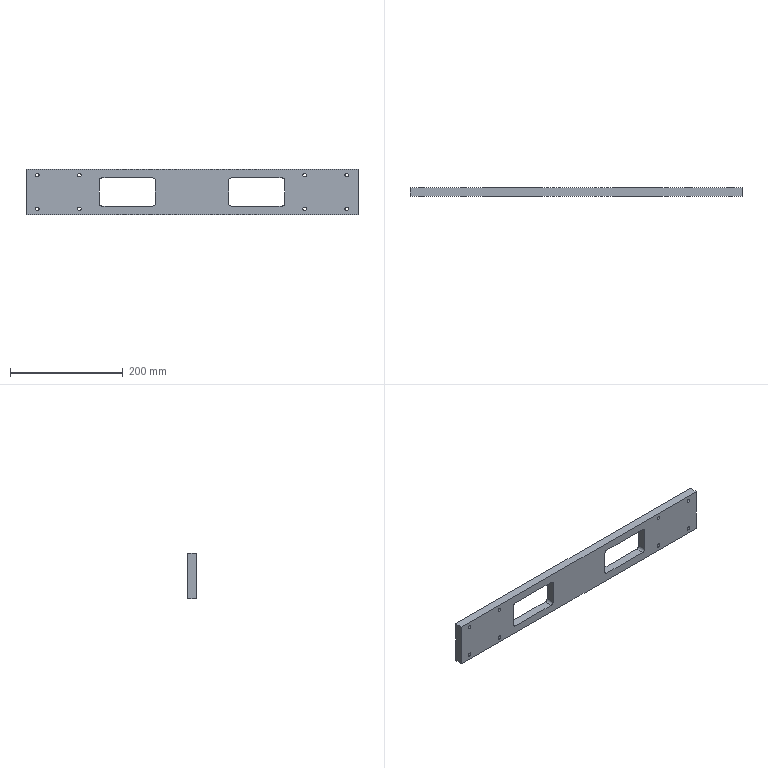Part | STEP file | 11-FG-SJ01011 | 1 solid | 62 faces | box 590 x 15 x 80 mm | volume 551424 mm3 | cylinder 40 | plane 22 | commonest cylinder face diameters 6.6 x16 11 x16 10 x8